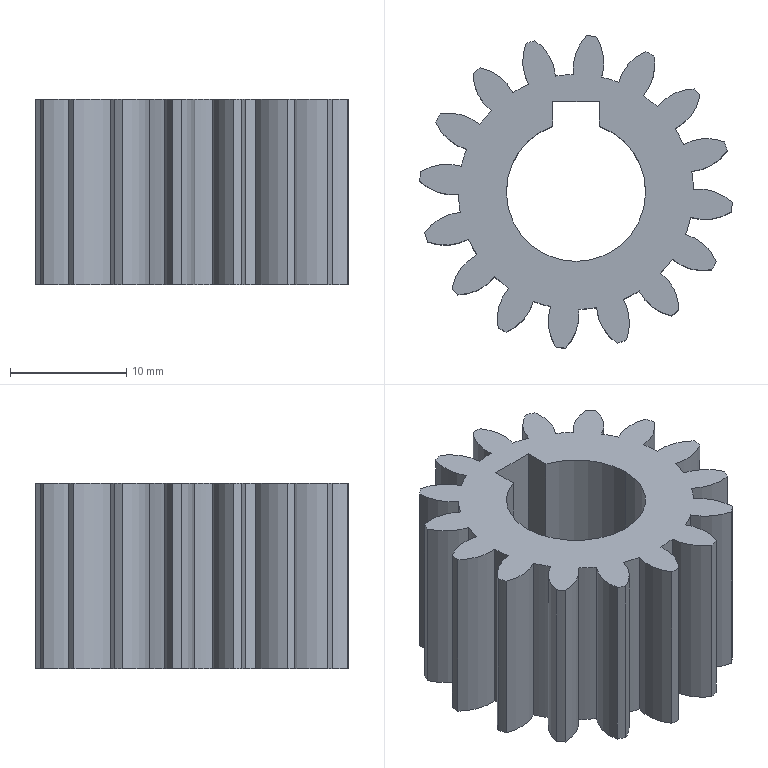Part | SolidWorks | features ICE 2, CirPattern 1, Extrusion 1 | 1 solid | 76 faces | box 26.937 x 26.937 x 16 mm | volume 5099 mm3 | cylinder 71 | plane 5 | commonest cylinder face diameters 8.208 x36 20.25 x16 27 x16 12 x3